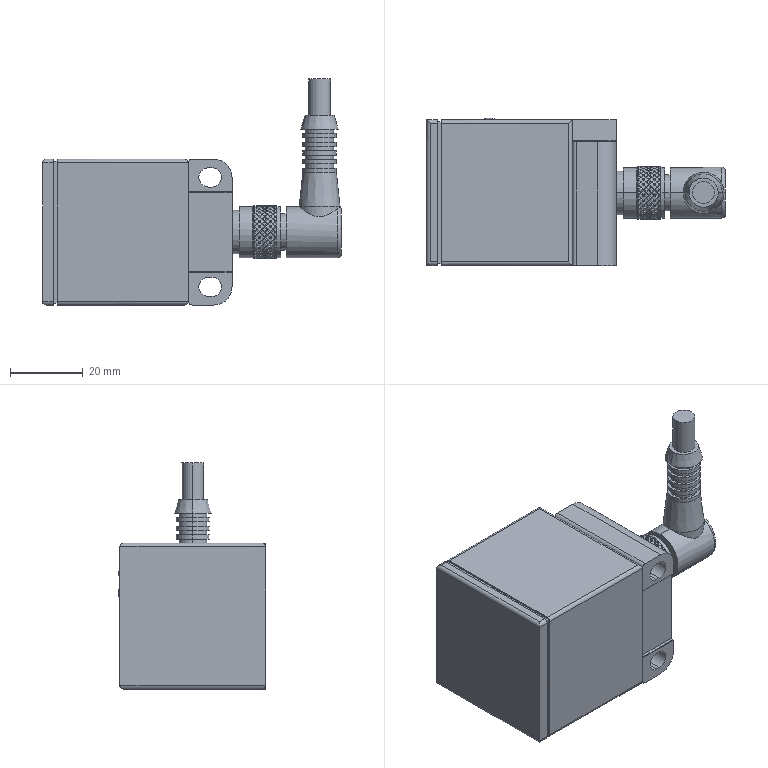Part | SolidWorks | 4 solids | 1814 faces | box 82 x 40.45 x 62 mm | volume 85684 mm3 | spline 1206 | cylinder 354 | plane 236 | cone 18 | commonest cylinder face diameters 14.5 x275 2 x14 1 x10 7.8 x10 9.2 x10 14 x6